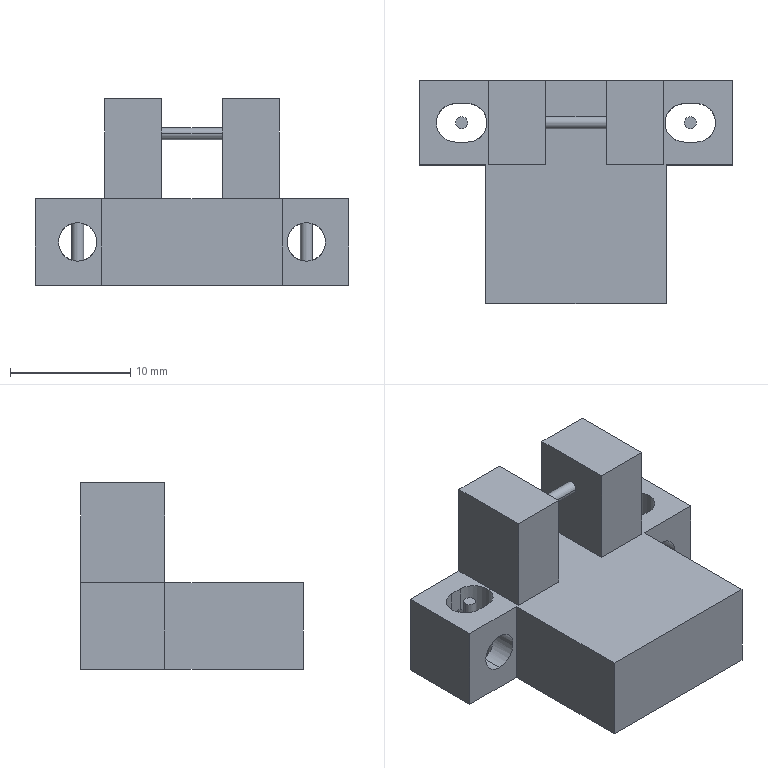Part | SolidWorks | features ICE 3, Extrusion 1, HoleWzd 1 | 3 solids | 50 faces | box 26 x 18.5 x 15.5 mm | volume 2894 mm3 | plane 30 | cylinder 20 | commonest cylinder face diameters 3.2 x14 1 x6